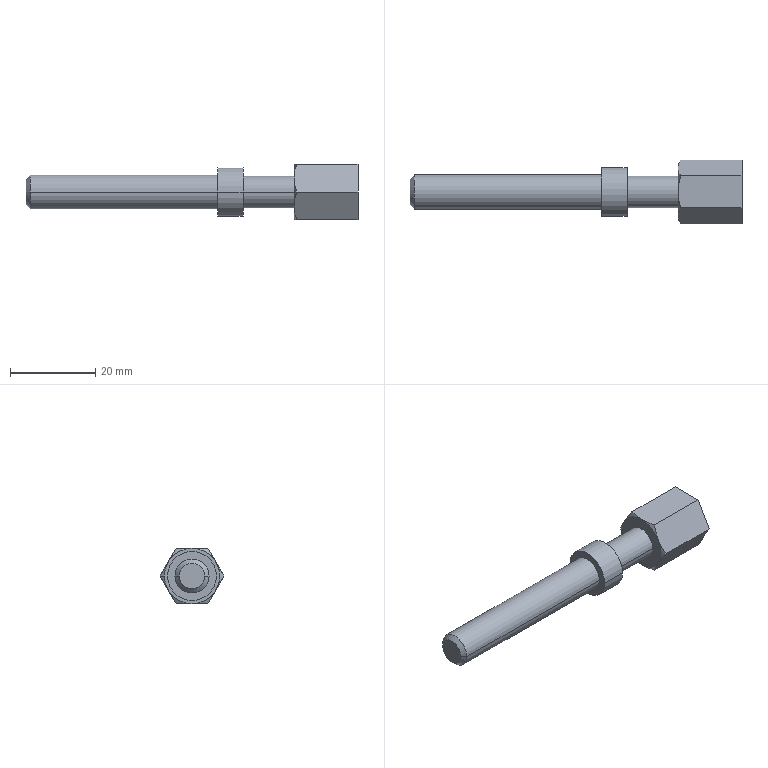Part | STEP file | AJSTS8-45 | 1 solid | 26 faces | box 78 x 15.011 x 13 mm | volume 5597 mm3 | plane 11 | cone 9 | cylinder 6 | commonest cylinder face diameters 7.5 x2 8 x2 11.5 x2
STEP:
#1=CARTESIAN_POINT('',(0.,-3.,0.));
#2=VERTEX_POINT('',#1);
#3=CARTESIAN_POINT('',(0.,3.,0.));
#4=VERTEX_POINT('',#3);
#5=CARTESIAN_POINT('',(0.,0.,0.));
#6=DIRECTION('',(-1.,0.,0.));
#7=DIRECTION('',(0.,1.,0.));
#8=AXIS2_PLACEMENT_3D('',#5,#6,#7);
#9=CIRCLE('',#8,3.);
#10=EDGE_CURVE('',#2,#4,#9,.T.);
#11=ORIENTED_EDGE('',*,*,#10,.F.);
#12=CARTESIAN_POINT('',(1.,-4.,0.));
#13=VERTEX_POINT('',#12);
#14=CARTESIAN_POINT('',(0.,-3.,0.));
#15=DIRECTION('',(0.7071,-0.7071,0.));
#16=VECTOR('',#15,1000.);
#17=LINE('',#14,#16);
#18=EDGE_CURVE('',#2,#13,#17,.T.);
#19=ORIENTED_EDGE('',*,*,#18,.T.);
#20=CARTESIAN_POINT('',(1.,4.,0.));
#21=VERTEX_POINT('',#20);
#22=CARTESIAN_POINT('',(1.,0.,0.));
#23=DIRECTION('',(1.,0.,0.));
#24=DIRECTION('',(0.,1.,0.));
#25=AXIS2_PLACEMENT_3D('',#22,#23,#24);
#26=CIRCLE('',#25,4.);
#27=EDGE_CURVE('',#21,#13,#26,.T.);
#28=ORIENTED_EDGE('',*,*,#27,.F.);
#29=CARTESIAN_POINT('',(0.,3.,0.));
#30=DIRECTION('',(0.7071,0.7071,0.));
#31=VECTOR('',#30,1000.);
#32=LINE('',#29,#31);
#33=EDGE_CURVE('',#4,#21,#32,.T.);
#34=ORIENTED_EDGE('',*,*,#33,.F.);
#35=EDGE_LOOP('',(#11,#19,#28,#34));
#36=FACE_OUTER_BOUND('',#35,.T.);
#37=CARTESIAN_POINT('',(0.,0.,0.));
#38=DIRECTION('',(1.,0.,0.));
#39=DIRECTION('',(0.,1.,0.));
#40=AXIS2_PLACEMENT_3D('',#37,#38,#39);
#41=CONICAL_SURFACE('',#40,3.,0.7854);
#42=ADVANCED_FACE('',(#36),#41,.T.);
#43=CARTESIAN_POINT('',(63.,6.5,0.));
#44=VERTEX_POINT('',#43);
#45=CARTESIAN_POINT('',(63.,5.629,-3.25));
#46=VERTEX_POINT('',#45);
#47=CARTESIAN_POINT('',(63.,0.,0.));
#48=DIRECTION('',(-1.,0.,0.));
#49=DIRECTION('',(0.,-1.,0.));
#50=AXIS2_PLACEMENT_3D('',#47,#48,#49);
#51=CIRCLE('',#50,6.5);
#52=EDGE_CURVE('',#44,#46,#51,.T.);
#53=ORIENTED_EDGE('',*,*,#52,.F.);
#54=CARTESIAN_POINT('',(63.581,7.506,0.));
#55=VERTEX_POINT('',#54);
#56=CARTESIAN_POINT('',(63.,6.5,0.));
#57=DIRECTION('',(0.5,0.866,0.));
#58=VECTOR('',#57,1000.);
#59=LINE('',#56,#58);
#60=EDGE_CURVE('',#44,#55,#59,.T.);
#61=ORIENTED_EDGE('',*,*,#60,.T.);
#62=CARTESIAN_POINT('',(63.581,7.506,0.));
#63=CARTESIAN_POINT('',(63.403,7.199,-0.5317));
#64=CARTESIAN_POINT('',(63.257,6.889,-1.067));
#65=CARTESIAN_POINT('',(63.055,6.265,-2.149));
#66=CARTESIAN_POINT('',(63.,5.949,-2.696));
#67=CARTESIAN_POINT('',(63.,5.629,-3.25));
#68=B_SPLINE_CURVE_WITH_KNOTS('',3,(#62,#63,#64,#65,#66,#67),.UNSPECIFIED.,.F.,.F.,(4,2,4),(0.000000238,0.001899,0.003797),.UNSPECIFIED.);
#69=EDGE_CURVE('',#55,#46,#68,.T.);
#70=ORIENTED_EDGE('',*,*,#69,.T.);
#71=EDGE_LOOP('',(#53,#61,#70));
#72=FACE_OUTER_BOUND('',#71,.T.);
#73=CARTESIAN_POINT('',(63.,0.,0.));
#74=DIRECTION('',(1.,0.,0.));
#75=DIRECTION('',(0.,1.,0.));
#76=AXIS2_PLACEMENT_3D('',#73,#74,#75);
#77=CONICAL_SURFACE('',#76,6.5,1.047);
#78=ADVANCED_FACE('',(#72),#77,.T.);
#79=CARTESIAN_POINT('',(63.,3.75,0.));
#80=VERTEX_POINT('',#79);
#81=CARTESIAN_POINT('',(63.,-3.75,0.));
#82=VERTEX_POINT('',#81);
#83=CARTESIAN_POINT('',(63.,0.,0.));
#84=DIRECTION('',(1.,0.,0.));
#85=DIRECTION('',(0.,0.,-1.));
#86=AXIS2_PLACEMENT_3D('',#83,#84,#85);
#87=CIRCLE('',#86,3.75);
#88=EDGE_CURVE('',#80,#82,#87,.T.);
#89=ORIENTED_EDGE('',*,*,#88,.F.);
#90=CARTESIAN_POINT('',(51.,3.75,0.));
#91=VERTEX_POINT('',#90);
#92=CARTESIAN_POINT('',(0.,3.75,0.));
#93=DIRECTION('',(-1.,0.,0.));
#94=VECTOR('',#93,1000.);
#95=LINE('',#92,#94);
#96=EDGE_CURVE('',#80,#91,#95,.T.);
#97=ORIENTED_EDGE('',*,*,#96,.T.);
#98=CARTESIAN_POINT('',(51.,-3.75,0.));
#99=VERTEX_POINT('',#98);
#100=CARTESIAN_POINT('',(51.,0.,0.));
#101=DIRECTION('',(-1.,0.,0.));
#102=DIRECTION('',(0.,-1.,0.));
#103=AXIS2_PLACEMENT_3D('',#100,#101,#102);
#104=CIRCLE('',#103,3.75);
#105=EDGE_CURVE('',#99,#91,#104,.T.);
#106=ORIENTED_EDGE('',*,*,#105,.F.);
#107=CARTESIAN_POINT('',(0.,-3.75,0.));
#108=DIRECTION('',(-1.,0.,0.));
#109=VECTOR('',#108,1000.);
#110=LINE('',#107,#109);
#111=EDGE_CURVE('',#82,#99,#110,.T.);
#112=ORIENTED_EDGE('',*,*,#111,.F.);
#113=EDGE_LOOP('',(#89,#97,#106,#112));
#114=FACE_OUTER_BOUND('',#113,.T.);
#115=CARTESIAN_POINT('',(0.,0.,0.));
#116=DIRECTION('',(-1.,0.,0.));
#117=DIRECTION('',(0.,-1.,0.));
#118=AXIS2_PLACEMENT_3D('',#115,#116,#117);
#119=CYLINDRICAL_SURFACE('',#118,3.75);
#120=ADVANCED_FACE('',(#114),#119,.T.);
#121=CARTESIAN_POINT('',(51.,-5.75,0.));
#122=VERTEX_POINT('',#121);
#123=CARTESIAN_POINT('',(51.,5.75,0.));
#124=VERTEX_POINT('',#123);
#125=CARTESIAN_POINT('',(51.,0.,0.));
#126=DIRECTION('',(-1.,0.,0.));
#127=DIRECTION('',(0.,-1.,0.));
#128=AXIS2_PLACEMENT_3D('',#125,#126,#127);
#129=CIRCLE('',#128,5.75);
#130=EDGE_CURVE('',#122,#124,#129,.T.);
#131=ORIENTED_EDGE('',*,*,#130,.T.);
#132=CARTESIAN_POINT('',(45.,5.75,0.));
#133=VERTEX_POINT('',#132);
#134=CARTESIAN_POINT('',(0.,5.75,0.));
#135=DIRECTION('',(-1.,0.,0.));
#136=VECTOR('',#135,1000.);
#137=LINE('',#134,#136);
#138=EDGE_CURVE('',#124,#133,#137,.T.);
#139=ORIENTED_EDGE('',*,*,#138,.T.);
#140=CARTESIAN_POINT('',(45.,-5.75,0.));
#141=VERTEX_POINT('',#140);
#142=CARTESIAN_POINT('',(45.,0.,0.));
#143=DIRECTION('',(-1.,0.,0.));
#144=DIRECTION('',(0.,-1.,0.));
#145=AXIS2_PLACEMENT_3D('',#142,#143,#144);
#146=CIRCLE('',#145,5.75);
#147=EDGE_CURVE('',#141,#133,#146,.T.);
#148=ORIENTED_EDGE('',*,*,#147,.F.);
#149=CARTESIAN_POINT('',(0.,-5.75,0.));
#150=DIRECTION('',(-1.,0.,0.));
#151=VECTOR('',#150,1000.);
#152=LINE('',#149,#151);
#153=EDGE_CURVE('',#122,#141,#152,.T.);
#154=ORIENTED_EDGE('',*,*,#153,.F.);
#155=EDGE_LOOP('',(#131,#139,#148,#154));
#156=FACE_OUTER_BOUND('',#155,.T.);
#157=CARTESIAN_POINT('',(0.,0.,0.));
#158=DIRECTION('',(-1.,0.,0.));
#159=DIRECTION('',(0.,-1.,0.));
#160=AXIS2_PLACEMENT_3D('',#157,#158,#159);
#161=CYLINDRICAL_SURFACE('',#160,5.75);
#162=ADVANCED_FACE('',(#156),#161,.T.);
#163=CARTESIAN_POINT('',(45.,-4.,0.));
#164=VERTEX_POINT('',#163);
#165=CARTESIAN_POINT('',(45.,4.,0.));
#166=VERTEX_POINT('',#165);
#167=CARTESIAN_POINT('',(45.,0.,0.));
#168=DIRECTION('',(-1.,0.,0.));
#169=DIRECTION('',(0.,-1.,0.));
#170=AXIS2_PLACEMENT_3D('',#167,#168,#169);
#171=CIRCLE('',#170,4.);
#172=EDGE_CURVE('',#164,#166,#171,.T.);
#173=ORIENTED_EDGE('',*,*,#172,.T.);
#174=CARTESIAN_POINT('',(0.,4.,0.));
#175=DIRECTION('',(-1.,0.,0.));
#176=VECTOR('',#175,1000.);
#177=LINE('',#174,#176);
#178=EDGE_CURVE('',#166,#21,#177,.T.);
#179=ORIENTED_EDGE('',*,*,#178,.T.);
#180=ORIENTED_EDGE('',*,*,#27,.T.);
#181=CARTESIAN_POINT('',(0.,-4.,0.));
#182=DIRECTION('',(-1.,0.,0.));
#183=VECTOR('',#182,1000.);
#184=LINE('',#181,#183);
#185=EDGE_CURVE('',#164,#13,#184,.T.);
#186=ORIENTED_EDGE('',*,*,#185,.F.);
#187=EDGE_LOOP('',(#173,#179,#180,#186));
#188=FACE_OUTER_BOUND('',#187,.T.);
#189=CARTESIAN_POINT('',(0.,0.,0.));
#190=DIRECTION('',(-1.,0.,0.));
#191=DIRECTION('',(0.,-1.,0.));
#192=AXIS2_PLACEMENT_3D('',#189,#190,#191);
#193=CYLINDRICAL_SURFACE('',#192,4.);
#194=ADVANCED_FACE('',(#188),#193,.T.);
#195=CARTESIAN_POINT('',(63.,0.,0.));
#196=DIRECTION('',(1.,0.,0.));
#197=DIRECTION('',(0.,0.,-1.));
#198=AXIS2_PLACEMENT_3D('',#195,#196,#197);
#199=CIRCLE('',#198,3.75);
#200=EDGE_CURVE('',#82,#80,#199,.T.);
#201=ORIENTED_EDGE('',*,*,#200,.T.);
#202=ORIENTED_EDGE('',*,*,#88,.T.);
#203=EDGE_LOOP('',(#201,#202));
#204=FACE_BOUND('',#203,.T.);
#205=CARTESIAN_POINT('',(63.,0.,-6.5));
#206=VERTEX_POINT('',#205);
#207=CARTESIAN_POINT('',(63.,0.,0.));
#208=DIRECTION('',(-1.,0.,0.));
#209=DIRECTION('',(0.,-1.,0.));
#210=AXIS2_PLACEMENT_3D('',#207,#208,#209);
#211=CIRCLE('',#210,6.5);
#212=EDGE_CURVE('',#46,#206,#211,.T.);
#213=ORIENTED_EDGE('',*,*,#212,.T.);
#214=CARTESIAN_POINT('',(63.,-5.629,-3.25));
#215=VERTEX_POINT('',#214);
#216=CARTESIAN_POINT('',(63.,0.,0.));
#217=DIRECTION('',(-1.,0.,0.));
#218=DIRECTION('',(0.,-1.,0.));
#219=AXIS2_PLACEMENT_3D('',#216,#217,#218);
#220=CIRCLE('',#219,6.5);
#221=EDGE_CURVE('',#206,#215,#220,.T.);
#222=ORIENTED_EDGE('',*,*,#221,.T.);
#223=CARTESIAN_POINT('',(63.,-5.629,3.25));
#224=VERTEX_POINT('',#223);
#225=CARTESIAN_POINT('',(63.,0.,0.));
#226=DIRECTION('',(-1.,0.,0.));
#227=DIRECTION('',(0.,-1.,0.));
#228=AXIS2_PLACEMENT_3D('',#225,#226,#227);
#229=CIRCLE('',#228,6.5);
#230=EDGE_CURVE('',#215,#224,#229,.T.);
#231=ORIENTED_EDGE('',*,*,#230,.T.);
#232=CARTESIAN_POINT('',(63.,0.,6.5));
#233=VERTEX_POINT('',#232);
#234=CARTESIAN_POINT('',(63.,0.,0.));
#235=DIRECTION('',(-1.,0.,0.));
#236=DIRECTION('',(0.,-1.,0.));
#237=AXIS2_PLACEMENT_3D('',#234,#235,#236);
#238=CIRCLE('',#237,6.5);
#239=EDGE_CURVE('',#224,#233,#238,.T.);
#240=ORIENTED_EDGE('',*,*,#239,.T.);
#241=CARTESIAN_POINT('',(63.,5.629,3.25));
#242=VERTEX_POINT('',#241);
#243=CARTESIAN_POINT('',(63.,0.,0.));
#244=DIRECTION('',(-1.,0.,0.));
#245=DIRECTION('',(0.,-1.,0.));
#246=AXIS2_PLACEMENT_3D('',#243,#244,#245);
#247=CIRCLE('',#246,6.5);
#248=EDGE_CURVE('',#233,#242,#247,.T.);
#249=ORIENTED_EDGE('',*,*,#248,.T.);
#250=CARTESIAN_POINT('',(63.,0.,0.));
#251=DIRECTION('',(-1.,0.,0.));
#252=DIRECTION('',(0.,-1.,0.));
#253=AXIS2_PLACEMENT_3D('',#250,#251,#252);
#254=CIRCLE('',#253,6.5);
#255=EDGE_CURVE('',#242,#44,#254,.T.);
#256=ORIENTED_EDGE('',*,*,#255,.T.);
#257=ORIENTED_EDGE('',*,*,#52,.T.);
#258=EDGE_LOOP('',(#213,#222,#231,#240,#249,#256,#257));
#259=FACE_OUTER_BOUND('',#258,.T.);
#260=CARTESIAN_POINT('',(63.,0.,0.));
#261=DIRECTION('',(1.,0.,0.));
#262=DIRECTION('',(0.,0.,-1.));
#263=AXIS2_PLACEMENT_3D('',#260,#261,#262);
#264=PLANE('',#263);
#265=ADVANCED_FACE('',(#204,#259),#264,.F.);
#266=CARTESIAN_POINT('',(0.,0.,0.));
#267=DIRECTION('',(-1.,0.,0.));
#268=DIRECTION('',(0.,1.,0.));
#269=AXIS2_PLACEMENT_3D('',#266,#267,#268);
#270=CIRCLE('',#269,3.);
#271=EDGE_CURVE('',#4,#2,#270,.T.);
#272=ORIENTED_EDGE('',*,*,#271,.T.);
#273=ORIENTED_EDGE('',*,*,#10,.T.);
#274=EDGE_LOOP('',(#272,#273));
#275=FACE_OUTER_BOUND('',#274,.T.);
#276=CARTESIAN_POINT('',(0.,0.,0.));
#277=DIRECTION('',(1.,0.,0.));
#278=DIRECTION('',(0.,1.,0.));
#279=AXIS2_PLACEMENT_3D('',#276,#277,#278);
#280=PLANE('',#279);
#281=ADVANCED_FACE('',(#275),#280,.F.);
#282=ORIENTED_EDGE('',*,*,#178,.F.);
#283=CARTESIAN_POINT('',(45.,0.,0.));
#284=DIRECTION('',(-1.,0.,0.));
#285=DIRECTION('',(0.,-1.,0.));
#286=AXIS2_PLACEMENT_3D('',#283,#284,#285);
#287=CIRCLE('',#286,4.);
#288=EDGE_CURVE('',#166,#164,#287,.T.);
#289=ORIENTED_EDGE('',*,*,#288,.T.);
#290=ORIENTED_EDGE('',*,*,#185,.T.);
#291=CARTESIAN_POINT('',(1.,0.,0.));
#292=DIRECTION('',(1.,0.,0.));
#293=DIRECTION('',(0.,1.,0.));
#294=AXIS2_PLACEMENT_3D('',#291,#292,#293);
#295=CIRCLE('',#294,4.);
#296=EDGE_CURVE('',#13,#21,#295,.T.);
#297=ORIENTED_EDGE('',*,*,#296,.T.);
#298=EDGE_LOOP('',(#282,#289,#290,#297));
#299=FACE_OUTER_BOUND('',#298,.T.);
#300=CARTESIAN_POINT('',(0.,0.,0.));
#301=DIRECTION('',(-1.,0.,0.));
#302=DIRECTION('',(0.,-1.,0.));
#303=AXIS2_PLACEMENT_3D('',#300,#301,#302);
#304=CYLINDRICAL_SURFACE('',#303,4.);
#305=ADVANCED_FACE('',(#299),#304,.T.);
#306=ORIENTED_EDGE('',*,*,#172,.F.);
#307=ORIENTED_EDGE('',*,*,#288,.F.);
#308=EDGE_LOOP('',(#306,#307));
#309=FACE_BOUND('',#308,.T.);
#310=ORIENTED_EDGE('',*,*,#147,.T.);
#311=CARTESIAN_POINT('',(45.,0.,0.));
#312=DIRECTION('',(-1.,0.,0.));
#313=DIRECTION('',(0.,-1.,0.));
#314=AXIS2_PLACEMENT_3D('',#311,#312,#313);
#315=CIRCLE('',#314,5.75);
#316=EDGE_CURVE('',#133,#141,#315,.T.);
#317=ORIENTED_EDGE('',*,*,#316,.T.);
#318=EDGE_LOOP('',(#310,#317));
#319=FACE_OUTER_BOUND('',#318,.T.);
#320=CARTESIAN_POINT('',(45.,4.,0.));
#321=DIRECTION('',(1.,0.,0.));
#322=DIRECTION('',(0.,1.,0.));
#323=AXIS2_PLACEMENT_3D('',#320,#321,#322);
#324=PLANE('',#323);
#325=ADVANCED_FACE('',(#309,#319),#324,.F.);
#326=ORIENTED_EDGE('',*,*,#138,.F.);
#327=CARTESIAN_POINT('',(51.,0.,0.));
#328=DIRECTION('',(-1.,0.,0.));
#329=DIRECTION('',(0.,-1.,0.));
#330=AXIS2_PLACEMENT_3D('',#327,#328,#329);
#331=CIRCLE('',#330,5.75);
#332=EDGE_CURVE('',#124,#122,#331,.T.);
#333=ORIENTED_EDGE('',*,*,#332,.T.);
#334=ORIENTED_EDGE('',*,*,#153,.T.);
#335=ORIENTED_EDGE('',*,*,#316,.F.);
#336=EDGE_LOOP('',(#326,#333,#334,#335));
#337=FACE_OUTER_BOUND('',#336,.T.);
#338=CARTESIAN_POINT('',(0.,0.,0.));
#339=DIRECTION('',(-1.,0.,0.));
#340=DIRECTION('',(0.,-1.,0.));
#341=AXIS2_PLACEMENT_3D('',#338,#339,#340);
#342=CYLINDRICAL_SURFACE('',#341,5.75);
#343=ADVANCED_FACE('',(#337),#342,.T.);
#344=ORIENTED_EDGE('',*,*,#130,.F.);
#345=ORIENTED_EDGE('',*,*,#332,.F.);
#346=EDGE_LOOP('',(#344,#345));
#347=FACE_OUTER_BOUND('',#346,.T.);
#348=ORIENTED_EDGE('',*,*,#105,.T.);
#349=CARTESIAN_POINT('',(51.,0.,0.));
#350=DIRECTION('',(-1.,0.,0.));
#351=DIRECTION('',(0.,-1.,0.));
#352=AXIS2_PLACEMENT_3D('',#349,#350,#351);
#353=CIRCLE('',#352,3.75);
#354=EDGE_CURVE('',#91,#99,#353,.T.);
#355=ORIENTED_EDGE('',*,*,#354,.T.);
#356=EDGE_LOOP('',(#348,#355));
#357=FACE_BOUND('',#356,.T.);
#358=CARTESIAN_POINT('',(51.,5.75,0.));
#359=DIRECTION('',(-1.,0.,0.));
#360=DIRECTION('',(0.,-1.,0.));
#361=AXIS2_PLACEMENT_3D('',#358,#359,#360);
#362=PLANE('',#361);
#363=ADVANCED_FACE('',(#347,#357),#362,.F.);
#364=ORIENTED_EDGE('',*,*,#96,.F.);
#365=ORIENTED_EDGE('',*,*,#200,.F.);
#366=ORIENTED_EDGE('',*,*,#111,.T.);
#367=ORIENTED_EDGE('',*,*,#354,.F.);
#368=EDGE_LOOP('',(#364,#365,#366,#367));
#369=FACE_OUTER_BOUND('',#368,.T.);
#370=CARTESIAN_POINT('',(0.,0.,0.));
#371=DIRECTION('',(-1.,0.,0.));
#372=DIRECTION('',(0.,-1.,0.));
#373=AXIS2_PLACEMENT_3D('',#370,#371,#372);
#374=CYLINDRICAL_SURFACE('',#373,3.75);
#375=ADVANCED_FACE('',(#369),#374,.T.);
#376=CARTESIAN_POINT('',(63.581,-3.753,6.5));
#377=VERTEX_POINT('',#376);
#378=CARTESIAN_POINT('',(63.581,-3.753,6.5));
#379=CARTESIAN_POINT('',(63.404,-3.142,6.5));
#380=CARTESIAN_POINT('',(63.257,-2.517,6.5));
#381=CARTESIAN_POINT('',(63.055,-1.264,6.5));
#382=CARTESIAN_POINT('',(63.,-0.6342,6.5));
#383=CARTESIAN_POINT('',(63.,0.,6.5));
#384=B_SPLINE_CURVE_WITH_KNOTS('',3,(#378,#379,#380,#381,#382,#383),.UNSPECIFIED.,.F.,.F.,(4,2,4),(0.006695,0.008594,0.01049),.UNSPECIFIED.);
#385=EDGE_CURVE('',#377,#233,#384,.T.);
#386=ORIENTED_EDGE('',*,*,#385,.T.);
#387=ORIENTED_EDGE('',*,*,#239,.F.);
#388=CARTESIAN_POINT('',(63.,-5.629,3.25));
#389=CARTESIAN_POINT('',(63.,-5.47,3.526));
#390=CARTESIAN_POINT('',(63.014,-5.31,3.803));
#391=CARTESIAN_POINT('',(63.067,-4.994,4.351));
#392=CARTESIAN_POINT('',(63.106,-4.836,4.623));
#393=CARTESIAN_POINT('',(63.258,-4.368,5.435));
#394=CARTESIAN_POINT('',(63.404,-4.059,5.97));
#395=CARTESIAN_POINT('',(63.581,-3.753,6.5));
#396=B_SPLINE_CURVE_WITH_KNOTS('',3,(#388,#389,#390,#391,#392,#393,#394,#395),.UNSPECIFIED.,.F.,.F.,(4,2,2,4),(0.003797,0.004743,0.005689,0.00758),.UNSPECIFIED.);
#397=EDGE_CURVE('',#224,#377,#396,.T.);
#398=ORIENTED_EDGE('',*,*,#397,.T.);
#399=EDGE_LOOP('',(#386,#387,#398));
#400=FACE_OUTER_BOUND('',#399,.T.);
#401=CARTESIAN_POINT('',(63.,0.,0.));
#402=DIRECTION('',(1.,0.,0.));
#403=DIRECTION('',(0.,1.,0.));
#404=AXIS2_PLACEMENT_3D('',#401,#402,#403);
#405=CONICAL_SURFACE('',#404,6.5,1.047);
#406=ADVANCED_FACE('',(#400),#405,.T.);
#407=CARTESIAN_POINT('',(63.581,-7.506,0.));
#408=VERTEX_POINT('',#407);
#409=CARTESIAN_POINT('',(63.,-5.629,-3.25));
#410=CARTESIAN_POINT('',(63.,-5.788,-2.974));
#411=CARTESIAN_POINT('',(63.014,-5.948,-2.697));
#412=CARTESIAN_POINT('',(63.067,-6.265,-2.149));
#413=CARTESIAN_POINT('',(63.106,-6.422,-1.877));
#414=CARTESIAN_POINT('',(63.258,-6.891,-1.065));
#415=CARTESIAN_POINT('',(63.404,-7.199,-0.5303));
#416=CARTESIAN_POINT('',(63.581,-7.506,0.));
#417=B_SPLINE_CURVE_WITH_KNOTS('',3,(#409,#410,#411,#412,#413,#414,#415,#416),.UNSPECIFIED.,.F.,.F.,(4,2,2,4),(0.003797,0.004743,0.005689,0.00758),.UNSPECIFIED.);
#418=EDGE_CURVE('',#215,#408,#417,.T.);
#419=ORIENTED_EDGE('',*,*,#418,.T.);
#420=CARTESIAN_POINT('',(63.581,-7.506,0.));
#421=CARTESIAN_POINT('',(63.403,-7.199,0.5317));
#422=CARTESIAN_POINT('',(63.257,-6.889,1.067));
#423=CARTESIAN_POINT('',(63.055,-6.265,2.149));
#424=CARTESIAN_POINT('',(63.,-5.949,2.696));
#425=CARTESIAN_POINT('',(63.,-5.629,3.25));
#426=B_SPLINE_CURVE_WITH_KNOTS('',3,(#420,#421,#422,#423,#424,#425),.UNSPECIFIED.,.F.,.F.,(4,2,4),(0.000000238,0.001899,0.003797),.UNSPECIFIED.);
#427=EDGE_CURVE('',#408,#224,#426,.T.);
#428=ORIENTED_EDGE('',*,*,#427,.T.);
#429=ORIENTED_EDGE('',*,*,#230,.F.);
#430=EDGE_LOOP('',(#419,#428,#429));
#431=FACE_OUTER_BOUND('',#430,.T.);
#432=CARTESIAN_POINT('',(63.,0.,0.));
#433=DIRECTION('',(1.,0.,0.));
#434=DIRECTION('',(0.,1.,0.));
#435=AXIS2_PLACEMENT_3D('',#432,#433,#434);
#436=CONICAL_SURFACE('',#435,6.5,1.047);
#437=ADVANCED_FACE('',(#431),#436,.T.);
#438=CARTESIAN_POINT('',(63.581,3.753,6.5));
#439=VERTEX_POINT('',#438);
#440=CARTESIAN_POINT('',(63.581,3.753,6.5));
#441=CARTESIAN_POINT('',(63.403,4.06,5.968));
#442=CARTESIAN_POINT('',(63.257,4.369,5.433));
#443=CARTESIAN_POINT('',(63.055,4.994,4.351));
#444=CARTESIAN_POINT('',(63.,5.309,3.804));
#445=CARTESIAN_POINT('',(63.,5.629,3.25));
#446=B_SPLINE_CURVE_WITH_KNOTS('',3,(#440,#441,#442,#443,#444,#445),.UNSPECIFIED.,.F.,.F.,(4,2,4),(0.000000238,0.001899,0.003797),.UNSPECIFIED.);
#447=EDGE_CURVE('',#439,#242,#446,.T.);
#448=ORIENTED_EDGE('',*,*,#447,.T.);
#449=ORIENTED_EDGE('',*,*,#248,.F.);
#450=CARTESIAN_POINT('',(63.,0.,6.5));
#451=CARTESIAN_POINT('',(63.,0.6345,6.5));
#452=CARTESIAN_POINT('',(63.056,1.278,6.5));
#453=CARTESIAN_POINT('',(63.26,2.531,6.5));
#454=CARTESIAN_POINT('',(63.405,3.146,6.5));
#455=CARTESIAN_POINT('',(63.581,3.753,6.5));
#456=B_SPLINE_CURVE_WITH_KNOTS('',3,(#450,#451,#452,#453,#454,#455),.UNSPECIFIED.,.F.,.F.,(4,2,4),(0.01049,0.01239,0.01429),.UNSPECIFIED.);
#457=EDGE_CURVE('',#233,#439,#456,.T.);
#458=ORIENTED_EDGE('',*,*,#457,.T.);
#459=EDGE_LOOP('',(#448,#449,#458));
#460=FACE_OUTER_BOUND('',#459,.T.);
#461=CARTESIAN_POINT('',(63.,0.,0.));
#462=DIRECTION('',(1.,0.,0.));
#463=DIRECTION('',(0.,1.,0.));
#464=AXIS2_PLACEMENT_3D('',#461,#462,#463);
#465=CONICAL_SURFACE('',#464,6.5,1.047);
#466=ADVANCED_FACE('',(#460),#465,.T.);
#467=ORIENTED_EDGE('',*,*,#60,.F.);
#468=ORIENTED_EDGE('',*,*,#255,.F.);
#469=CARTESIAN_POINT('',(63.,5.629,3.25));
#470=CARTESIAN_POINT('',(63.,5.788,2.974));
#471=CARTESIAN_POINT('',(63.014,5.948,2.697));
#472=CARTESIAN_POINT('',(63.067,6.265,2.149));
#473=CARTESIAN_POINT('',(63.106,6.422,1.877));
#474=CARTESIAN_POINT('',(63.258,6.891,1.065));
#475=CARTESIAN_POINT('',(63.404,7.199,0.5303));
#476=CARTESIAN_POINT('',(63.581,7.506,0.));
#477=B_SPLINE_CURVE_WITH_KNOTS('',3,(#469,#470,#471,#472,#473,#474,#475,#476),.UNSPECIFIED.,.F.,.F.,(4,2,2,4),(0.003797,0.004743,0.005689,0.00758),.UNSPECIFIED.);
#478=EDGE_CURVE('',#242,#55,#477,.T.);
#479=ORIENTED_EDGE('',*,*,#478,.T.);
#480=EDGE_LOOP('',(#467,#468,#479));
#481=FACE_OUTER_BOUND('',#480,.T.);
#482=CARTESIAN_POINT('',(63.,0.,0.));
#483=DIRECTION('',(1.,0.,0.));
#484=DIRECTION('',(0.,1.,0.));
#485=AXIS2_PLACEMENT_3D('',#482,#483,#484);
#486=CONICAL_SURFACE('',#485,6.5,1.047);
#487=ADVANCED_FACE('',(#481),#486,.T.);
#488=CARTESIAN_POINT('',(63.581,3.753,-6.5));
#489=VERTEX_POINT('',#488);
#490=CARTESIAN_POINT('',(63.,5.629,-3.25));
#491=CARTESIAN_POINT('',(63.,5.47,-3.526));
#492=CARTESIAN_POINT('',(63.014,5.31,-3.803));
#493=CARTESIAN_POINT('',(63.067,4.994,-4.351));
#494=CARTESIAN_POINT('',(63.106,4.836,-4.623));
#495=CARTESIAN_POINT('',(63.258,4.368,-5.435));
#496=CARTESIAN_POINT('',(63.404,4.059,-5.97));
#497=CARTESIAN_POINT('',(63.581,3.753,-6.5));
#498=B_SPLINE_CURVE_WITH_KNOTS('',3,(#490,#491,#492,#493,#494,#495,#496,#497),.UNSPECIFIED.,.F.,.F.,(4,2,2,4),(0.003797,0.004743,0.005689,0.00758),.UNSPECIFIED.);
#499=EDGE_CURVE('',#46,#489,#498,.T.);
#500=ORIENTED_EDGE('',*,*,#499,.T.);
#501=CARTESIAN_POINT('',(63.581,3.753,-6.5));
#502=CARTESIAN_POINT('',(63.405,3.146,-6.5));
#503=CARTESIAN_POINT('',(63.26,2.531,-6.5));
#504=CARTESIAN_POINT('',(63.056,1.278,-6.5));
#505=CARTESIAN_POINT('',(63.,0.6345,-6.5));
#506=CARTESIAN_POINT('',(63.,0.,-6.5));
#507=B_SPLINE_CURVE_WITH_KNOTS('',3,(#501,#502,#503,#504,#505,#506),.UNSPECIFIED.,.F.,.F.,(4,2,4),(0.002751,0.004645,0.00654),.UNSPECIFIED.);
#508=EDGE_CURVE('',#489,#206,#507,.T.);
#509=ORIENTED_EDGE('',*,*,#508,.T.);
#510=ORIENTED_EDGE('',*,*,#212,.F.);
#511=EDGE_LOOP('',(#500,#509,#510));
#512=FACE_OUTER_BOUND('',#511,.T.);
#513=CARTESIAN_POINT('',(63.,0.,0.));
#514=DIRECTION('',(1.,0.,0.));
#515=DIRECTION('',(0.,1.,0.));
#516=AXIS2_PLACEMENT_3D('',#513,#514,#515);
#517=CONICAL_SURFACE('',#516,6.5,1.047);
#518=ADVANCED_FACE('',(#512),#517,.T.);
#519=CARTESIAN_POINT('',(63.581,-3.753,-6.5));
#520=VERTEX_POINT('',#519);
#521=CARTESIAN_POINT('',(63.,0.,-6.5));
#522=CARTESIAN_POINT('',(63.,-0.6342,-6.5));
#523=CARTESIAN_POINT('',(63.055,-1.264,-6.5));
#524=CARTESIAN_POINT('',(63.257,-2.517,-6.5));
#525=CARTESIAN_POINT('',(63.404,-3.142,-6.5));
#526=CARTESIAN_POINT('',(63.581,-3.753,-6.5));
#527=B_SPLINE_CURVE_WITH_KNOTS('',3,(#521,#522,#523,#524,#525,#526),.UNSPECIFIED.,.F.,.F.,(4,2,4),(0.00654,0.008433,0.01033),.UNSPECIFIED.);
#528=EDGE_CURVE('',#206,#520,#527,.T.);
#529=ORIENTED_EDGE('',*,*,#528,.T.);
#530=CARTESIAN_POINT('',(63.581,-3.753,-6.5));
#531=CARTESIAN_POINT('',(63.403,-4.06,-5.968));
#532=CARTESIAN_POINT('',(63.257,-4.369,-5.433));
#533=CARTESIAN_POINT('',(63.055,-4.994,-4.351));
#534=CARTESIAN_POINT('',(63.,-5.309,-3.804));
#535=CARTESIAN_POINT('',(63.,-5.629,-3.25));
#536=B_SPLINE_CURVE_WITH_KNOTS('',3,(#530,#531,#532,#533,#534,#535),.UNSPECIFIED.,.F.,.F.,(4,2,4),(0.000000238,0.001899,0.003797),.UNSPECIFIED.);
#537=EDGE_CURVE('',#520,#215,#536,.T.);
#538=ORIENTED_EDGE('',*,*,#537,.T.);
#539=ORIENTED_EDGE('',*,*,#221,.F.);
#540=EDGE_LOOP('',(#529,#538,#539));
#541=FACE_OUTER_BOUND('',#540,.T.);
#542=CARTESIAN_POINT('',(63.,0.,0.));
#543=DIRECTION('',(1.,0.,0.));
#544=DIRECTION('',(0.,1.,0.));
#545=AXIS2_PLACEMENT_3D('',#542,#543,#544);
#546=CONICAL_SURFACE('',#545,6.5,1.047);
#547=ADVANCED_FACE('',(#541),#546,.T.);
#548=CARTESIAN_POINT('',(78.,-7.506,0.));
#549=VERTEX_POINT('',#548);
#550=CARTESIAN_POINT('',(78.,-3.753,-6.5));
#551=VERTEX_POINT('',#550);
#552=CARTESIAN_POINT('',(78.,-7.506,0.));
#553=DIRECTION('',(0.,0.5,-0.866));
#554=VECTOR('',#553,1000.);
#555=LINE('',#552,#554);
#556=EDGE_CURVE('',#549,#551,#555,.T.);
#557=ORIENTED_EDGE('',*,*,#556,.T.);
#558=CARTESIAN_POINT('',(78.,3.753,-6.5));
#559=VERTEX_POINT('',#558);
#560=CARTESIAN_POINT('',(78.,-3.753,-6.5));
#561=DIRECTION('',(0.,1.,0.));
#562=VECTOR('',#561,1000.);
#563=LINE('',#560,#562);
#564=EDGE_CURVE('',#551,#559,#563,.T.);
#565=ORIENTED_EDGE('',*,*,#564,.T.);
#566=CARTESIAN_POINT('',(78.,7.506,0.));
#567=VERTEX_POINT('',#566);
#568=CARTESIAN_POINT('',(78.,3.753,-6.5));
#569=DIRECTION('',(0.,0.5,0.866));
#570=VECTOR('',#569,1000.);
#571=LINE('',#568,#570);
#572=EDGE_CURVE('',#559,#567,#571,.T.);
#573=ORIENTED_EDGE('',*,*,#572,.T.);
#574=CARTESIAN_POINT('',(78.,3.753,6.5));
#575=VERTEX_POINT('',#574);
#576=CARTESIAN_POINT('',(78.,7.506,0.));
#577=DIRECTION('',(0.,-0.5,0.866));
#578=VECTOR('',#577,1000.);
#579=LINE('',#576,#578);
#580=EDGE_CURVE('',#567,#575,#579,.T.);
#581=ORIENTED_EDGE('',*,*,#580,.T.);
#582=CARTESIAN_POINT('',(78.,-3.753,6.5));
#583=VERTEX_POINT('',#582);
#584=CARTESIAN_POINT('',(78.,3.753,6.5));
#585=DIRECTION('',(0.,-1.,0.));
#586=VECTOR('',#585,1000.);
#587=LINE('',#584,#586);
#588=EDGE_CURVE('',#575,#583,#587,.T.);
#589=ORIENTED_EDGE('',*,*,#588,.T.);
#590=CARTESIAN_POINT('',(78.,-3.753,6.5));
#591=DIRECTION('',(0.,-0.5,-0.866));
#592=VECTOR('',#591,1000.);
#593=LINE('',#590,#592);
#594=EDGE_CURVE('',#583,#549,#593,.T.);
#595=ORIENTED_EDGE('',*,*,#594,.T.);
#596=EDGE_LOOP('',(#557,#565,#573,#581,#589,#595));
#597=FACE_OUTER_BOUND('',#596,.T.);
#598=CARTESIAN_POINT('',(78.,0.,0.));
#599=DIRECTION('',(1.,0.,0.));
#600=DIRECTION('',(0.,0.,-1.));
#601=AXIS2_PLACEMENT_3D('',#598,#599,#600);
#602=PLANE('',#601);
#603=ADVANCED_FACE('',(#597),#602,.T.);
#604=ORIENTED_EDGE('',*,*,#427,.F.);
#605=CARTESIAN_POINT('',(78.,-7.506,0.));
#606=DIRECTION('',(-1.,0.,0.));
#607=VECTOR('',#606,1000.);
#608=LINE('',#605,#607);
#609=EDGE_CURVE('',#549,#408,#608,.T.);
#610=ORIENTED_EDGE('',*,*,#609,.F.);
#611=ORIENTED_EDGE('',*,*,#594,.F.);
#612=CARTESIAN_POINT('',(78.,-3.753,6.5));
#613=DIRECTION('',(-1.,0.,0.));
#614=VECTOR('',#613,1000.);
#615=LINE('',#612,#614);
#616=EDGE_CURVE('',#583,#377,#615,.T.);
#617=ORIENTED_EDGE('',*,*,#616,.T.);
#618=ORIENTED_EDGE('',*,*,#397,.F.);
#619=EDGE_LOOP('',(#604,#610,#611,#617,#618));
#620=FACE_OUTER_BOUND('',#619,.T.);
#621=CARTESIAN_POINT('',(78.,-3.753,6.5));
#622=DIRECTION('',(0.,0.866,-0.5));
#623=DIRECTION('',(0.,0.5,0.866));
#624=AXIS2_PLACEMENT_3D('',#621,#622,#623);
#625=PLANE('',#624);
#626=ADVANCED_FACE('',(#620),#625,.F.);
#627=ORIENTED_EDGE('',*,*,#385,.F.);
#628=ORIENTED_EDGE('',*,*,#616,.F.);
#629=ORIENTED_EDGE('',*,*,#588,.F.);
#630=CARTESIAN_POINT('',(78.,3.753,6.5));
#631=DIRECTION('',(-1.,0.,0.));
#632=VECTOR('',#631,1000.);
#633=LINE('',#630,#632);
#634=EDGE_CURVE('',#575,#439,#633,.T.);
#635=ORIENTED_EDGE('',*,*,#634,.T.);
#636=ORIENTED_EDGE('',*,*,#457,.F.);
#637=EDGE_LOOP('',(#627,#628,#629,#635,#636));
#638=FACE_OUTER_BOUND('',#637,.T.);
#639=CARTESIAN_POINT('',(78.,3.753,6.5));
#640=DIRECTION('',(0.,0.,-1.));
#641=DIRECTION('',(-1.,0.,0.));
#642=AXIS2_PLACEMENT_3D('',#639,#640,#641);
#643=PLANE('',#642);
#644=ADVANCED_FACE('',(#638),#643,.F.);
#645=ORIENTED_EDGE('',*,*,#447,.F.);
#646=ORIENTED_EDGE('',*,*,#634,.F.);
#647=ORIENTED_EDGE('',*,*,#580,.F.);
#648=CARTESIAN_POINT('',(78.,7.506,0.));
#649=DIRECTION('',(-1.,0.,0.));
#650=VECTOR('',#649,1000.);
#651=LINE('',#648,#650);
#652=EDGE_CURVE('',#567,#55,#651,.T.);
#653=ORIENTED_EDGE('',*,*,#652,.T.);
#654=ORIENTED_EDGE('',*,*,#478,.F.);
#655=EDGE_LOOP('',(#645,#646,#647,#653,#654));
#656=FACE_OUTER_BOUND('',#655,.T.);
#657=CARTESIAN_POINT('',(78.,7.506,0.));
#658=DIRECTION('',(0.,-0.866,-0.5));
#659=DIRECTION('',(0.,0.5,-0.866));
#660=AXIS2_PLACEMENT_3D('',#657,#658,#659);
#661=PLANE('',#660);
#662=ADVANCED_FACE('',(#656),#661,.F.);
#663=ORIENTED_EDGE('',*,*,#69,.F.);
#664=ORIENTED_EDGE('',*,*,#652,.F.);
#665=ORIENTED_EDGE('',*,*,#572,.F.);
#666=CARTESIAN_POINT('',(78.,3.753,-6.5));
#667=DIRECTION('',(-1.,0.,0.));
#668=VECTOR('',#667,1000.);
#669=LINE('',#666,#668);
#670=EDGE_CURVE('',#559,#489,#669,.T.);
#671=ORIENTED_EDGE('',*,*,#670,.T.);
#672=ORIENTED_EDGE('',*,*,#499,.F.);
#673=EDGE_LOOP('',(#663,#664,#665,#671,#672));
#674=FACE_OUTER_BOUND('',#673,.T.);
#675=CARTESIAN_POINT('',(78.,3.753,-6.5));
#676=DIRECTION('',(0.,-0.866,0.5));
#677=DIRECTION('',(0.,-0.5,-0.866));
#678=AXIS2_PLACEMENT_3D('',#675,#676,#677);
#679=PLANE('',#678);
#680=ADVANCED_FACE('',(#674),#679,.F.);
#681=ORIENTED_EDGE('',*,*,#508,.F.);
#682=ORIENTED_EDGE('',*,*,#670,.F.);
#683=ORIENTED_EDGE('',*,*,#564,.F.);
#684=CARTESIAN_POINT('',(78.,-3.753,-6.5));
#685=DIRECTION('',(-1.,0.,0.));
#686=VECTOR('',#685,1000.);
#687=LINE('',#684,#686);
#688=EDGE_CURVE('',#551,#520,#687,.T.);
#689=ORIENTED_EDGE('',*,*,#688,.T.);
#690=ORIENTED_EDGE('',*,*,#528,.F.);
#691=EDGE_LOOP('',(#681,#682,#683,#689,#690));
#692=FACE_OUTER_BOUND('',#691,.T.);
#693=CARTESIAN_POINT('',(78.,-3.753,-6.5));
#694=DIRECTION('',(0.,0.,1.));
#695=DIRECTION('',(0.,-1.,0.));
#696=AXIS2_PLACEMENT_3D('',#693,#694,#695);
#697=PLANE('',#696);
#698=ADVANCED_FACE('',(#692),#697,.F.);
#699=ORIENTED_EDGE('',*,*,#537,.F.);
#700=ORIENTED_EDGE('',*,*,#688,.F.);
#701=ORIENTED_EDGE('',*,*,#556,.F.);
#702=ORIENTED_EDGE('',*,*,#609,.T.);
#703=ORIENTED_EDGE('',*,*,#418,.F.);
#704=EDGE_LOOP('',(#699,#700,#701,#702,#703));
#705=FACE_OUTER_BOUND('',#704,.T.);
#706=CARTESIAN_POINT('',(78.,-7.506,0.));
#707=DIRECTION('',(0.,0.866,0.5));
#708=DIRECTION('',(0.,-0.5,0.866));
#709=AXIS2_PLACEMENT_3D('',#706,#707,#708);
#710=PLANE('',#709);
#711=ADVANCED_FACE('',(#705),#710,.F.);
#712=ORIENTED_EDGE('',*,*,#18,.F.);
#713=ORIENTED_EDGE('',*,*,#271,.F.);
#714=ORIENTED_EDGE('',*,*,#33,.T.);
#715=ORIENTED_EDGE('',*,*,#296,.F.);
#716=EDGE_LOOP('',(#712,#713,#714,#715));
#717=FACE_OUTER_BOUND('',#716,.T.);
#718=CARTESIAN_POINT('',(0.,0.,0.));
#719=DIRECTION('',(1.,0.,0.));
#720=DIRECTION('',(0.,1.,0.));
#721=AXIS2_PLACEMENT_3D('',#718,#719,#720);
#722=CONICAL_SURFACE('',#721,3.,0.7854);
#723=ADVANCED_FACE('',(#717),#722,.T.);
#724=CLOSED_SHELL('',(#42,#78,#120,#162,#194,#265,#281,#305,#325,#343,#363,#375,#406,#437,#466,#487,#518,#547,#603,#626,#644,#662,#680,#698,#711,#723));
#725=MANIFOLD_SOLID_BREP('',#724);
#726=CARTESIAN_POINT('',(0.,0.,0.));
#727=DIRECTION('',(0.,0.,1.));
#728=DIRECTION('',(1.,0.,0.));
#729=AXIS2_PLACEMENT_3D('',#726,#727,#728);
#730=(LENGTH_UNIT()NAMED_UNIT(*)SI_UNIT(.MILLI.,.METRE.));
#731=UNCERTAINTY_MEASURE_WITH_UNIT(LENGTH_MEASURE(0.00001),#730,'','');
#732=(NAMED_UNIT(*)PLANE_ANGLE_UNIT()SI_UNIT($,.RADIAN.));
#733=(NAMED_UNIT(*)SI_UNIT($,.STERADIAN.)SOLID_ANGLE_UNIT());
#734=(GEOMETRIC_REPRESENTATION_CONTEXT(3)GLOBAL_UNCERTAINTY_ASSIGNED_CONTEXT((#731))GLOBAL_UNIT_ASSIGNED_CONTEXT((#730,#732,#733))REPRESENTATION_CONTEXT('',''));
#735=ADVANCED_BREP_SHAPE_REPRESENTATION('',(#725,#729),#734);